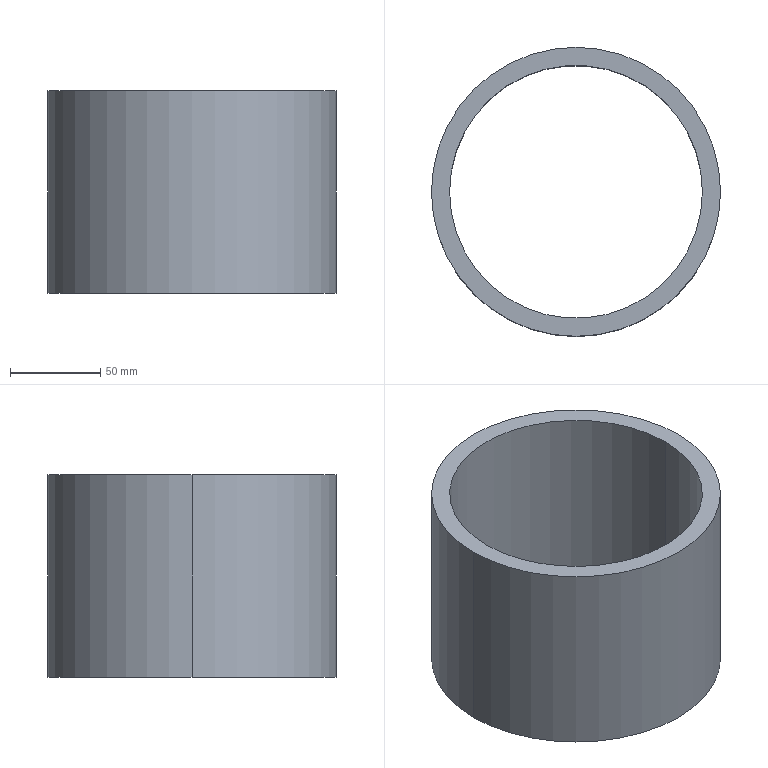Part | NX | features BREP 1 | 1 solid | 6 faces | box 160 x 160 x 112 mm | volume 527788 mm3 | cylinder 4 | plane 2 | commonest cylinder face diameters 140 x2 160 x2
STEP:
#1=CARTESIAN_POINT('',(-70.,0.,112.));
#2=VERTEX_POINT('',#1);
#3=CARTESIAN_POINT('',(70.,0.,112.));
#4=VERTEX_POINT('',#3);
#5=CARTESIAN_POINT('',(0.,0.,112.));
#6=DIRECTION('',(0.,0.,1.));
#7=DIRECTION('',(1.,0.,0.));
#8=AXIS2_PLACEMENT_3D('',#5,#6,#7);
#9=CIRCLE('',#8,70.);
#10=EDGE_CURVE('',#2,#4,#9,.T.);
#11=ORIENTED_EDGE('',*,*,#10,.T.);
#12=CARTESIAN_POINT('',(70.,0.,0.));
#13=VERTEX_POINT('',#12);
#14=CARTESIAN_POINT('',(70.,0.,112.));
#15=DIRECTION('',(0.,0.,-1.));
#16=VECTOR('',#15,1000.);
#17=LINE('',#14,#16);
#18=EDGE_CURVE('',#13,#4,#17,.F.);
#19=ORIENTED_EDGE('',*,*,#18,.F.);
#20=CARTESIAN_POINT('',(-70.,0.,0.));
#21=VERTEX_POINT('',#20);
#22=CARTESIAN_POINT('',(0.,0.,0.));
#23=DIRECTION('',(0.,0.,1.));
#24=DIRECTION('',(1.,0.,0.));
#25=AXIS2_PLACEMENT_3D('',#22,#23,#24);
#26=CIRCLE('',#25,70.);
#27=EDGE_CURVE('',#21,#13,#26,.T.);
#28=ORIENTED_EDGE('',*,*,#27,.F.);
#29=CARTESIAN_POINT('',(-70.,0.,112.));
#30=DIRECTION('',(0.,0.,-1.));
#31=VECTOR('',#30,1000.);
#32=LINE('',#29,#31);
#33=EDGE_CURVE('',#21,#2,#32,.F.);
#34=ORIENTED_EDGE('',*,*,#33,.T.);
#35=EDGE_LOOP('',(#11,#19,#28,#34));
#36=FACE_BOUND('',#35,.T.);
#37=CARTESIAN_POINT('',(0.,0.,112.));
#38=DIRECTION('',(0.,0.,-1.));
#39=DIRECTION('',(1.,0.,0.));
#40=AXIS2_PLACEMENT_3D('',#37,#38,#39);
#41=CYLINDRICAL_SURFACE('',#40,70.);
#42=ADVANCED_FACE('',(#36),#41,.F.);
#43=CARTESIAN_POINT('',(80.,0.,112.));
#44=VERTEX_POINT('',#43);
#45=CARTESIAN_POINT('',(-80.,0.,112.));
#46=VERTEX_POINT('',#45);
#47=CARTESIAN_POINT('',(0.,0.,112.));
#48=DIRECTION('',(0.,0.,1.));
#49=DIRECTION('',(1.,0.,0.));
#50=AXIS2_PLACEMENT_3D('',#47,#48,#49);
#51=CIRCLE('',#50,80.);
#52=EDGE_CURVE('',#44,#46,#51,.T.);
#53=ORIENTED_EDGE('',*,*,#52,.F.);
#54=CARTESIAN_POINT('',(80.,0.,0.));
#55=VERTEX_POINT('',#54);
#56=CARTESIAN_POINT('',(80.,0.,112.));
#57=DIRECTION('',(0.,0.,-1.));
#58=VECTOR('',#57,1000.);
#59=LINE('',#56,#58);
#60=EDGE_CURVE('',#55,#44,#59,.F.);
#61=ORIENTED_EDGE('',*,*,#60,.F.);
#62=CARTESIAN_POINT('',(-80.,0.,0.));
#63=VERTEX_POINT('',#62);
#64=CARTESIAN_POINT('',(0.,0.,0.));
#65=DIRECTION('',(0.,0.,1.));
#66=DIRECTION('',(1.,0.,0.));
#67=AXIS2_PLACEMENT_3D('',#64,#65,#66);
#68=CIRCLE('',#67,80.);
#69=EDGE_CURVE('',#55,#63,#68,.T.);
#70=ORIENTED_EDGE('',*,*,#69,.T.);
#71=CARTESIAN_POINT('',(-80.,0.,112.));
#72=DIRECTION('',(0.,0.,-1.));
#73=VECTOR('',#72,1000.);
#74=LINE('',#71,#73);
#75=EDGE_CURVE('',#63,#46,#74,.F.);
#76=ORIENTED_EDGE('',*,*,#75,.T.);
#77=EDGE_LOOP('',(#53,#61,#70,#76));
#78=FACE_BOUND('',#77,.T.);
#79=CARTESIAN_POINT('',(0.,0.,112.));
#80=DIRECTION('',(0.,0.,-1.));
#81=DIRECTION('',(1.,0.,0.));
#82=AXIS2_PLACEMENT_3D('',#79,#80,#81);
#83=CYLINDRICAL_SURFACE('',#82,80.);
#84=ADVANCED_FACE('',(#78),#83,.T.);
#85=CARTESIAN_POINT('',(0.,0.,112.));
#86=DIRECTION('',(0.,0.,1.));
#87=DIRECTION('',(1.,0.,0.));
#88=AXIS2_PLACEMENT_3D('',#85,#86,#87);
#89=CIRCLE('',#88,80.);
#90=EDGE_CURVE('',#46,#44,#89,.T.);
#91=ORIENTED_EDGE('',*,*,#90,.T.);
#92=ORIENTED_EDGE('',*,*,#52,.T.);
#93=EDGE_LOOP('',(#91,#92));
#94=FACE_BOUND('',#93,.T.);
#95=ORIENTED_EDGE('',*,*,#10,.F.);
#96=CARTESIAN_POINT('',(0.,0.,112.));
#97=DIRECTION('',(0.,0.,1.));
#98=DIRECTION('',(1.,0.,0.));
#99=AXIS2_PLACEMENT_3D('',#96,#97,#98);
#100=CIRCLE('',#99,70.);
#101=EDGE_CURVE('',#4,#2,#100,.T.);
#102=ORIENTED_EDGE('',*,*,#101,.F.);
#103=EDGE_LOOP('',(#95,#102));
#104=FACE_BOUND('',#103,.T.);
#105=CARTESIAN_POINT('',(0.,0.,112.));
#106=DIRECTION('',(0.,0.,1.));
#107=DIRECTION('',(-1.,0.,0.));
#108=AXIS2_PLACEMENT_3D('',#105,#106,#107);
#109=PLANE('',#108);
#110=ADVANCED_FACE('',(#94,#104),#109,.T.);
#111=CARTESIAN_POINT('',(0.,0.,0.));
#112=DIRECTION('',(0.,0.,1.));
#113=DIRECTION('',(1.,0.,0.));
#114=AXIS2_PLACEMENT_3D('',#111,#112,#113);
#115=CIRCLE('',#114,80.);
#116=EDGE_CURVE('',#63,#55,#115,.T.);
#117=ORIENTED_EDGE('',*,*,#116,.F.);
#118=ORIENTED_EDGE('',*,*,#69,.F.);
#119=EDGE_LOOP('',(#117,#118));
#120=FACE_BOUND('',#119,.T.);
#121=ORIENTED_EDGE('',*,*,#27,.T.);
#122=CARTESIAN_POINT('',(0.,0.,0.));
#123=DIRECTION('',(0.,0.,1.));
#124=DIRECTION('',(1.,0.,0.));
#125=AXIS2_PLACEMENT_3D('',#122,#123,#124);
#126=CIRCLE('',#125,70.);
#127=EDGE_CURVE('',#13,#21,#126,.T.);
#128=ORIENTED_EDGE('',*,*,#127,.T.);
#129=EDGE_LOOP('',(#121,#128));
#130=FACE_BOUND('',#129,.T.);
#131=CARTESIAN_POINT('',(0.,0.,0.));
#132=DIRECTION('',(0.,0.,1.));
#133=DIRECTION('',(-1.,0.,0.));
#134=AXIS2_PLACEMENT_3D('',#131,#132,#133);
#135=PLANE('',#134);
#136=ADVANCED_FACE('',(#120,#130),#135,.F.);
#137=ORIENTED_EDGE('',*,*,#60,.T.);
#138=ORIENTED_EDGE('',*,*,#90,.F.);
#139=ORIENTED_EDGE('',*,*,#75,.F.);
#140=ORIENTED_EDGE('',*,*,#116,.T.);
#141=EDGE_LOOP('',(#137,#138,#139,#140));
#142=FACE_BOUND('',#141,.T.);
#143=CARTESIAN_POINT('',(0.,0.,112.));
#144=DIRECTION('',(0.,0.,-1.));
#145=DIRECTION('',(1.,0.,0.));
#146=AXIS2_PLACEMENT_3D('',#143,#144,#145);
#147=CYLINDRICAL_SURFACE('',#146,80.);
#148=ADVANCED_FACE('',(#142),#147,.T.);
#149=ORIENTED_EDGE('',*,*,#18,.T.);
#150=ORIENTED_EDGE('',*,*,#101,.T.);
#151=ORIENTED_EDGE('',*,*,#33,.F.);
#152=ORIENTED_EDGE('',*,*,#127,.F.);
#153=EDGE_LOOP('',(#149,#150,#151,#152));
#154=FACE_BOUND('',#153,.T.);
#155=CARTESIAN_POINT('',(0.,0.,112.));
#156=DIRECTION('',(0.,0.,-1.));
#157=DIRECTION('',(1.,0.,0.));
#158=AXIS2_PLACEMENT_3D('',#155,#156,#157);
#159=CYLINDRICAL_SURFACE('',#158,70.);
#160=ADVANCED_FACE('',(#154),#159,.F.);
#161=CLOSED_SHELL('',(#42,#84,#110,#136,#148,#160));
#162=MANIFOLD_SOLID_BREP('',#161);
#163=(LENGTH_UNIT()NAMED_UNIT(*)SI_UNIT(.MILLI.,.METRE.));
#164=UNCERTAINTY_MEASURE_WITH_UNIT(LENGTH_MEASURE(0.00001),#163,'','');
#165=(NAMED_UNIT(*)PLANE_ANGLE_UNIT()SI_UNIT($,.RADIAN.));
#166=(NAMED_UNIT(*)SI_UNIT($,.STERADIAN.)SOLID_ANGLE_UNIT());
#167=(GEOMETRIC_REPRESENTATION_CONTEXT(3)GLOBAL_UNCERTAINTY_ASSIGNED_CONTEXT((#164))GLOBAL_UNIT_ASSIGNED_CONTEXT((#163,#165,#166))REPRESENTATION_CONTEXT('',''));
#168=ADVANCED_BREP_SHAPE_REPRESENTATION('',(#162),#167);